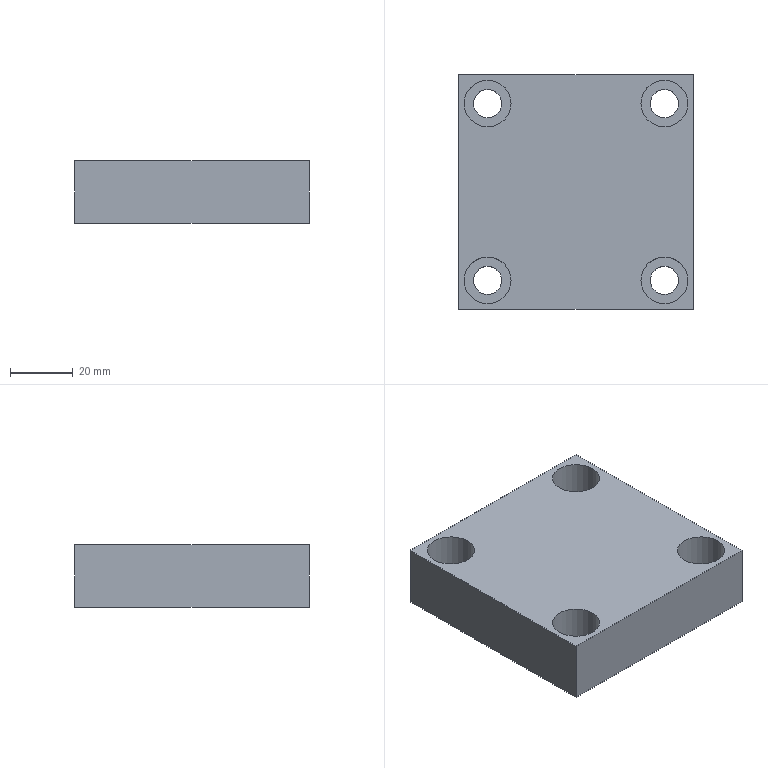Part | NX | features solid 2 | 1 solid | 18 faces | box 75 x 75 x 20 mm | volume 101982 mm3 | plane 10 | cylinder 8 | commonest cylinder face diameters 9 x4 15 x4
STEP:
#1=CARTESIAN_POINT('',(131.25,551.75,290.));
#2=VERTEX_POINT('',#1);
#3=CARTESIAN_POINT('',(126.75,551.75,290.));
#4=DIRECTION('',(0.,0.,1.));
#5=DIRECTION('',(1.,0.,0.));
#6=AXIS2_PLACEMENT_3D('',#3,#4,#5);
#7=CIRCLE('',#6,4.5);
#8=EDGE_CURVE('',#2,#2,#7,.T.);
#9=ORIENTED_EDGE('',*,*,#8,.T.);
#10=EDGE_LOOP('',(#9));
#11=FACE_BOUND('',#10,.T.);
#12=CARTESIAN_POINT('',(187.75,551.75,290.));
#13=VERTEX_POINT('',#12);
#14=CARTESIAN_POINT('',(183.25,551.75,290.));
#15=DIRECTION('',(0.,0.,1.));
#16=DIRECTION('',(1.,0.,0.));
#17=AXIS2_PLACEMENT_3D('',#14,#15,#16);
#18=CIRCLE('',#17,4.5);
#19=EDGE_CURVE('',#13,#13,#18,.T.);
#20=ORIENTED_EDGE('',*,*,#19,.T.);
#21=EDGE_LOOP('',(#20));
#22=FACE_BOUND('',#21,.T.);
#23=CARTESIAN_POINT('',(187.75,608.25,290.));
#24=VERTEX_POINT('',#23);
#25=CARTESIAN_POINT('',(183.25,608.25,290.));
#26=DIRECTION('',(0.,0.,1.));
#27=DIRECTION('',(1.,0.,0.));
#28=AXIS2_PLACEMENT_3D('',#25,#26,#27);
#29=CIRCLE('',#28,4.5);
#30=EDGE_CURVE('',#24,#24,#29,.T.);
#31=ORIENTED_EDGE('',*,*,#30,.T.);
#32=EDGE_LOOP('',(#31));
#33=FACE_BOUND('',#32,.T.);
#34=CARTESIAN_POINT('',(131.25,608.25,290.));
#35=VERTEX_POINT('',#34);
#36=CARTESIAN_POINT('',(126.75,608.25,290.));
#37=DIRECTION('',(0.,0.,1.));
#38=DIRECTION('',(1.,0.,0.));
#39=AXIS2_PLACEMENT_3D('',#36,#37,#38);
#40=CIRCLE('',#39,4.5);
#41=EDGE_CURVE('',#35,#35,#40,.T.);
#42=ORIENTED_EDGE('',*,*,#41,.T.);
#43=EDGE_LOOP('',(#42));
#44=FACE_BOUND('',#43,.T.);
#45=CARTESIAN_POINT('',(192.5,542.5,290.));
#46=VERTEX_POINT('',#45);
#47=CARTESIAN_POINT('',(117.5,542.5,290.));
#48=VERTEX_POINT('',#47);
#49=CARTESIAN_POINT('',(192.5,542.5,290.));
#50=DIRECTION('',(1.,0.,0.));
#51=VECTOR('',#50,1000.);
#52=LINE('',#49,#51);
#53=EDGE_CURVE('',#46,#48,#52,.F.);
#54=ORIENTED_EDGE('',*,*,#53,.T.);
#55=CARTESIAN_POINT('',(117.5,617.5,290.));
#56=VERTEX_POINT('',#55);
#57=CARTESIAN_POINT('',(117.5,630.,290.));
#58=DIRECTION('',(0.,-1.,0.));
#59=VECTOR('',#58,1000.);
#60=LINE('',#57,#59);
#61=EDGE_CURVE('',#56,#48,#60,.T.);
#62=ORIENTED_EDGE('',*,*,#61,.F.);
#63=CARTESIAN_POINT('',(192.5,617.5,290.));
#64=VERTEX_POINT('',#63);
#65=CARTESIAN_POINT('',(192.5,617.5,290.));
#66=DIRECTION('',(-1.,0.,0.));
#67=VECTOR('',#66,1000.);
#68=LINE('',#65,#67);
#69=EDGE_CURVE('',#64,#56,#68,.T.);
#70=ORIENTED_EDGE('',*,*,#69,.F.);
#71=CARTESIAN_POINT('',(192.5,630.,290.));
#72=DIRECTION('',(0.,1.,0.));
#73=VECTOR('',#72,1000.);
#74=LINE('',#71,#73);
#75=EDGE_CURVE('',#64,#46,#74,.F.);
#76=ORIENTED_EDGE('',*,*,#75,.T.);
#77=EDGE_LOOP('',(#54,#62,#70,#76));
#78=FACE_BOUND('',#77,.T.);
#79=CARTESIAN_POINT('',(192.5,630.,290.));
#80=DIRECTION('',(0.,0.,-1.));
#81=DIRECTION('',(1.,0.,0.));
#82=AXIS2_PLACEMENT_3D('',#79,#80,#81);
#83=PLANE('',#82);
#84=ADVANCED_FACE('',(#11,#22,#33,#44,#78),#83,.T.);
#85=CARTESIAN_POINT('',(117.5,617.5,310.));
#86=VERTEX_POINT('',#85);
#87=CARTESIAN_POINT('',(117.5,617.5,290.));
#88=DIRECTION('',(0.,0.,1.));
#89=VECTOR('',#88,1000.);
#90=LINE('',#87,#89);
#91=EDGE_CURVE('',#56,#86,#90,.T.);
#92=ORIENTED_EDGE('',*,*,#91,.T.);
#93=CARTESIAN_POINT('',(192.5,617.5,310.));
#94=VERTEX_POINT('',#93);
#95=CARTESIAN_POINT('',(192.5,617.5,310.));
#96=DIRECTION('',(-1.,0.,0.));
#97=VECTOR('',#96,1000.);
#98=LINE('',#95,#97);
#99=EDGE_CURVE('',#94,#86,#98,.T.);
#100=ORIENTED_EDGE('',*,*,#99,.F.);
#101=CARTESIAN_POINT('',(192.5,617.5,290.));
#102=DIRECTION('',(0.,0.,-1.));
#103=VECTOR('',#102,1000.);
#104=LINE('',#101,#103);
#105=EDGE_CURVE('',#64,#94,#104,.F.);
#106=ORIENTED_EDGE('',*,*,#105,.F.);
#107=ORIENTED_EDGE('',*,*,#69,.T.);
#108=EDGE_LOOP('',(#92,#100,#106,#107));
#109=FACE_BOUND('',#108,.T.);
#110=CARTESIAN_POINT('',(192.5,617.5,290.));
#111=DIRECTION('',(0.,1.,0.));
#112=DIRECTION('',(-1.,0.,0.));
#113=AXIS2_PLACEMENT_3D('',#110,#111,#112);
#114=PLANE('',#113);
#115=ADVANCED_FACE('',(#109),#114,.T.);
#116=ORIENTED_EDGE('',*,*,#105,.T.);
#117=CARTESIAN_POINT('',(192.5,542.5,310.));
#118=VERTEX_POINT('',#117);
#119=CARTESIAN_POINT('',(192.5,630.,310.));
#120=DIRECTION('',(0.,1.,0.));
#121=VECTOR('',#120,1000.);
#122=LINE('',#119,#121);
#123=EDGE_CURVE('',#94,#118,#122,.F.);
#124=ORIENTED_EDGE('',*,*,#123,.T.);
#125=CARTESIAN_POINT('',(192.5,542.5,290.));
#126=DIRECTION('',(0.,0.,1.));
#127=VECTOR('',#126,1000.);
#128=LINE('',#125,#127);
#129=EDGE_CURVE('',#46,#118,#128,.T.);
#130=ORIENTED_EDGE('',*,*,#129,.F.);
#131=ORIENTED_EDGE('',*,*,#75,.F.);
#132=EDGE_LOOP('',(#116,#124,#130,#131));
#133=FACE_BOUND('',#132,.T.);
#134=CARTESIAN_POINT('',(192.5,630.,290.));
#135=DIRECTION('',(-1.,0.,0.));
#136=DIRECTION('',(0.,-1.,0.));
#137=AXIS2_PLACEMENT_3D('',#134,#135,#136);
#138=PLANE('',#137);
#139=ADVANCED_FACE('',(#133),#138,.F.);
#140=ORIENTED_EDGE('',*,*,#129,.T.);
#141=CARTESIAN_POINT('',(117.5,542.5,310.));
#142=VERTEX_POINT('',#141);
#143=CARTESIAN_POINT('',(192.5,542.5,310.));
#144=DIRECTION('',(1.,0.,0.));
#145=VECTOR('',#144,1000.);
#146=LINE('',#143,#145);
#147=EDGE_CURVE('',#118,#142,#146,.F.);
#148=ORIENTED_EDGE('',*,*,#147,.T.);
#149=CARTESIAN_POINT('',(117.5,542.5,290.));
#150=DIRECTION('',(0.,0.,-1.));
#151=VECTOR('',#150,1000.);
#152=LINE('',#149,#151);
#153=EDGE_CURVE('',#48,#142,#152,.F.);
#154=ORIENTED_EDGE('',*,*,#153,.F.);
#155=ORIENTED_EDGE('',*,*,#53,.F.);
#156=EDGE_LOOP('',(#140,#148,#154,#155));
#157=FACE_BOUND('',#156,.T.);
#158=CARTESIAN_POINT('',(192.5,542.5,290.));
#159=DIRECTION('',(0.,1.,0.));
#160=DIRECTION('',(-1.,0.,0.));
#161=AXIS2_PLACEMENT_3D('',#158,#159,#160);
#162=PLANE('',#161);
#163=ADVANCED_FACE('',(#157),#162,.F.);
#164=ORIENTED_EDGE('',*,*,#61,.T.);
#165=ORIENTED_EDGE('',*,*,#153,.T.);
#166=CARTESIAN_POINT('',(117.5,630.,310.));
#167=DIRECTION('',(0.,-1.,0.));
#168=VECTOR('',#167,1000.);
#169=LINE('',#166,#168);
#170=EDGE_CURVE('',#86,#142,#169,.T.);
#171=ORIENTED_EDGE('',*,*,#170,.F.);
#172=ORIENTED_EDGE('',*,*,#91,.F.);
#173=EDGE_LOOP('',(#164,#165,#171,#172));
#174=FACE_BOUND('',#173,.T.);
#175=CARTESIAN_POINT('',(117.5,630.,290.));
#176=DIRECTION('',(-1.,0.,0.));
#177=DIRECTION('',(0.,-1.,0.));
#178=AXIS2_PLACEMENT_3D('',#175,#176,#177);
#179=PLANE('',#178);
#180=ADVANCED_FACE('',(#174),#179,.T.);
#181=CARTESIAN_POINT('',(134.25,551.75,310.));
#182=VERTEX_POINT('',#181);
#183=CARTESIAN_POINT('',(126.75,551.75,310.));
#184=DIRECTION('',(0.,0.,1.));
#185=DIRECTION('',(1.,0.,0.));
#186=AXIS2_PLACEMENT_3D('',#183,#184,#185);
#187=CIRCLE('',#186,7.5);
#188=EDGE_CURVE('',#182,#182,#187,.T.);
#189=ORIENTED_EDGE('',*,*,#188,.F.);
#190=EDGE_LOOP('',(#189));
#191=FACE_BOUND('',#190,.T.);
#192=CARTESIAN_POINT('',(190.75,551.75,310.));
#193=VERTEX_POINT('',#192);
#194=CARTESIAN_POINT('',(183.25,551.75,310.));
#195=DIRECTION('',(0.,0.,1.));
#196=DIRECTION('',(1.,0.,0.));
#197=AXIS2_PLACEMENT_3D('',#194,#195,#196);
#198=CIRCLE('',#197,7.5);
#199=EDGE_CURVE('',#193,#193,#198,.T.);
#200=ORIENTED_EDGE('',*,*,#199,.F.);
#201=EDGE_LOOP('',(#200));
#202=FACE_BOUND('',#201,.T.);
#203=CARTESIAN_POINT('',(190.75,608.25,310.));
#204=VERTEX_POINT('',#203);
#205=CARTESIAN_POINT('',(183.25,608.25,310.));
#206=DIRECTION('',(0.,0.,1.));
#207=DIRECTION('',(1.,0.,0.));
#208=AXIS2_PLACEMENT_3D('',#205,#206,#207);
#209=CIRCLE('',#208,7.5);
#210=EDGE_CURVE('',#204,#204,#209,.T.);
#211=ORIENTED_EDGE('',*,*,#210,.F.);
#212=EDGE_LOOP('',(#211));
#213=FACE_BOUND('',#212,.T.);
#214=CARTESIAN_POINT('',(134.25,608.25,310.));
#215=VERTEX_POINT('',#214);
#216=CARTESIAN_POINT('',(126.75,608.25,310.));
#217=DIRECTION('',(0.,0.,1.));
#218=DIRECTION('',(1.,0.,0.));
#219=AXIS2_PLACEMENT_3D('',#216,#217,#218);
#220=CIRCLE('',#219,7.5);
#221=EDGE_CURVE('',#215,#215,#220,.T.);
#222=ORIENTED_EDGE('',*,*,#221,.F.);
#223=EDGE_LOOP('',(#222));
#224=FACE_BOUND('',#223,.T.);
#225=ORIENTED_EDGE('',*,*,#147,.F.);
#226=ORIENTED_EDGE('',*,*,#123,.F.);
#227=ORIENTED_EDGE('',*,*,#99,.T.);
#228=ORIENTED_EDGE('',*,*,#170,.T.);
#229=EDGE_LOOP('',(#225,#226,#227,#228));
#230=FACE_BOUND('',#229,.T.);
#231=CARTESIAN_POINT('',(192.5,630.,310.));
#232=DIRECTION('',(0.,0.,-1.));
#233=DIRECTION('',(1.,0.,0.));
#234=AXIS2_PLACEMENT_3D('',#231,#232,#233);
#235=PLANE('',#234);
#236=ADVANCED_FACE('',(#191,#202,#213,#224,#230),#235,.F.);
#237=CARTESIAN_POINT('',(134.25,608.25,298.));
#238=VERTEX_POINT('',#237);
#239=CARTESIAN_POINT('',(126.75,608.25,298.));
#240=DIRECTION('',(0.,0.,-1.));
#241=DIRECTION('',(1.,0.,0.));
#242=AXIS2_PLACEMENT_3D('',#239,#240,#241);
#243=CIRCLE('',#242,7.5);
#244=EDGE_CURVE('',#238,#238,#243,.T.);
#245=ORIENTED_EDGE('',*,*,#244,.T.);
#246=EDGE_LOOP('',(#245));
#247=FACE_BOUND('',#246,.T.);
#248=ORIENTED_EDGE('',*,*,#221,.T.);
#249=EDGE_LOOP('',(#248));
#250=FACE_BOUND('',#249,.T.);
#251=CARTESIAN_POINT('',(126.75,608.25,298.));
#252=DIRECTION('',(0.,0.,1.));
#253=DIRECTION('',(-1.,0.,0.));
#254=AXIS2_PLACEMENT_3D('',#251,#252,#253);
#255=CYLINDRICAL_SURFACE('',#254,7.5);
#256=ADVANCED_FACE('',(#247,#250),#255,.F.);
#257=CARTESIAN_POINT('',(122.25,608.25,298.));
#258=VERTEX_POINT('',#257);
#259=CARTESIAN_POINT('',(126.75,608.25,298.));
#260=DIRECTION('',(0.,0.,-1.));
#261=DIRECTION('',(-1.,0.,0.));
#262=AXIS2_PLACEMENT_3D('',#259,#260,#261);
#263=CIRCLE('',#262,4.5);
#264=EDGE_CURVE('',#258,#258,#263,.T.);
#265=ORIENTED_EDGE('',*,*,#264,.T.);
#266=EDGE_LOOP('',(#265));
#267=FACE_BOUND('',#266,.T.);
#268=ORIENTED_EDGE('',*,*,#244,.F.);
#269=EDGE_LOOP('',(#268));
#270=FACE_BOUND('',#269,.T.);
#271=CARTESIAN_POINT('',(126.75,608.25,298.));
#272=DIRECTION('',(0.,0.,1.));
#273=DIRECTION('',(-1.,0.,0.));
#274=AXIS2_PLACEMENT_3D('',#271,#272,#273);
#275=PLANE('',#274);
#276=ADVANCED_FACE('',(#267,#270),#275,.T.);
#277=ORIENTED_EDGE('',*,*,#41,.F.);
#278=EDGE_LOOP('',(#277));
#279=FACE_BOUND('',#278,.T.);
#280=ORIENTED_EDGE('',*,*,#264,.F.);
#281=EDGE_LOOP('',(#280));
#282=FACE_BOUND('',#281,.T.);
#283=CARTESIAN_POINT('',(126.75,608.25,278.));
#284=DIRECTION('',(0.,0.,1.));
#285=DIRECTION('',(-1.,0.,0.));
#286=AXIS2_PLACEMENT_3D('',#283,#284,#285);
#287=CYLINDRICAL_SURFACE('',#286,4.5);
#288=ADVANCED_FACE('',(#279,#282),#287,.F.);
#289=CARTESIAN_POINT('',(190.75,608.25,298.));
#290=VERTEX_POINT('',#289);
#291=CARTESIAN_POINT('',(183.25,608.25,298.));
#292=DIRECTION('',(0.,0.,-1.));
#293=DIRECTION('',(1.,0.,0.));
#294=AXIS2_PLACEMENT_3D('',#291,#292,#293);
#295=CIRCLE('',#294,7.5);
#296=EDGE_CURVE('',#290,#290,#295,.T.);
#297=ORIENTED_EDGE('',*,*,#296,.T.);
#298=EDGE_LOOP('',(#297));
#299=FACE_BOUND('',#298,.T.);
#300=ORIENTED_EDGE('',*,*,#210,.T.);
#301=EDGE_LOOP('',(#300));
#302=FACE_BOUND('',#301,.T.);
#303=CARTESIAN_POINT('',(183.25,608.25,298.));
#304=DIRECTION('',(0.,0.,1.));
#305=DIRECTION('',(-1.,0.,0.));
#306=AXIS2_PLACEMENT_3D('',#303,#304,#305);
#307=CYLINDRICAL_SURFACE('',#306,7.5);
#308=ADVANCED_FACE('',(#299,#302),#307,.F.);
#309=CARTESIAN_POINT('',(178.75,608.25,298.));
#310=VERTEX_POINT('',#309);
#311=CARTESIAN_POINT('',(183.25,608.25,298.));
#312=DIRECTION('',(0.,0.,-1.));
#313=DIRECTION('',(-1.,0.,0.));
#314=AXIS2_PLACEMENT_3D('',#311,#312,#313);
#315=CIRCLE('',#314,4.5);
#316=EDGE_CURVE('',#310,#310,#315,.T.);
#317=ORIENTED_EDGE('',*,*,#316,.T.);
#318=EDGE_LOOP('',(#317));
#319=FACE_BOUND('',#318,.T.);
#320=ORIENTED_EDGE('',*,*,#296,.F.);
#321=EDGE_LOOP('',(#320));
#322=FACE_BOUND('',#321,.T.);
#323=CARTESIAN_POINT('',(183.25,608.25,298.));
#324=DIRECTION('',(0.,0.,1.));
#325=DIRECTION('',(-1.,0.,0.));
#326=AXIS2_PLACEMENT_3D('',#323,#324,#325);
#327=PLANE('',#326);
#328=ADVANCED_FACE('',(#319,#322),#327,.T.);
#329=ORIENTED_EDGE('',*,*,#30,.F.);
#330=EDGE_LOOP('',(#329));
#331=FACE_BOUND('',#330,.T.);
#332=ORIENTED_EDGE('',*,*,#316,.F.);
#333=EDGE_LOOP('',(#332));
#334=FACE_BOUND('',#333,.T.);
#335=CARTESIAN_POINT('',(183.25,608.25,278.));
#336=DIRECTION('',(0.,0.,1.));
#337=DIRECTION('',(-1.,0.,0.));
#338=AXIS2_PLACEMENT_3D('',#335,#336,#337);
#339=CYLINDRICAL_SURFACE('',#338,4.5);
#340=ADVANCED_FACE('',(#331,#334),#339,.F.);
#341=CARTESIAN_POINT('',(190.75,551.75,298.));
#342=VERTEX_POINT('',#341);
#343=CARTESIAN_POINT('',(183.25,551.75,298.));
#344=DIRECTION('',(0.,0.,-1.));
#345=DIRECTION('',(1.,0.,0.));
#346=AXIS2_PLACEMENT_3D('',#343,#344,#345);
#347=CIRCLE('',#346,7.5);
#348=EDGE_CURVE('',#342,#342,#347,.T.);
#349=ORIENTED_EDGE('',*,*,#348,.T.);
#350=EDGE_LOOP('',(#349));
#351=FACE_BOUND('',#350,.T.);
#352=ORIENTED_EDGE('',*,*,#199,.T.);
#353=EDGE_LOOP('',(#352));
#354=FACE_BOUND('',#353,.T.);
#355=CARTESIAN_POINT('',(183.25,551.75,298.));
#356=DIRECTION('',(0.,0.,1.));
#357=DIRECTION('',(-1.,0.,0.));
#358=AXIS2_PLACEMENT_3D('',#355,#356,#357);
#359=CYLINDRICAL_SURFACE('',#358,7.5);
#360=ADVANCED_FACE('',(#351,#354),#359,.F.);
#361=CARTESIAN_POINT('',(178.75,551.75,298.));
#362=VERTEX_POINT('',#361);
#363=CARTESIAN_POINT('',(183.25,551.75,298.));
#364=DIRECTION('',(0.,0.,-1.));
#365=DIRECTION('',(-1.,0.,0.));
#366=AXIS2_PLACEMENT_3D('',#363,#364,#365);
#367=CIRCLE('',#366,4.5);
#368=EDGE_CURVE('',#362,#362,#367,.T.);
#369=ORIENTED_EDGE('',*,*,#368,.T.);
#370=EDGE_LOOP('',(#369));
#371=FACE_BOUND('',#370,.T.);
#372=ORIENTED_EDGE('',*,*,#348,.F.);
#373=EDGE_LOOP('',(#372));
#374=FACE_BOUND('',#373,.T.);
#375=CARTESIAN_POINT('',(183.25,551.75,298.));
#376=DIRECTION('',(0.,0.,1.));
#377=DIRECTION('',(-1.,0.,0.));
#378=AXIS2_PLACEMENT_3D('',#375,#376,#377);
#379=PLANE('',#378);
#380=ADVANCED_FACE('',(#371,#374),#379,.T.);
#381=ORIENTED_EDGE('',*,*,#19,.F.);
#382=EDGE_LOOP('',(#381));
#383=FACE_BOUND('',#382,.T.);
#384=ORIENTED_EDGE('',*,*,#368,.F.);
#385=EDGE_LOOP('',(#384));
#386=FACE_BOUND('',#385,.T.);
#387=CARTESIAN_POINT('',(183.25,551.75,278.));
#388=DIRECTION('',(0.,0.,1.));
#389=DIRECTION('',(-1.,0.,0.));
#390=AXIS2_PLACEMENT_3D('',#387,#388,#389);
#391=CYLINDRICAL_SURFACE('',#390,4.5);
#392=ADVANCED_FACE('',(#383,#386),#391,.F.);
#393=CARTESIAN_POINT('',(134.25,551.75,298.));
#394=VERTEX_POINT('',#393);
#395=CARTESIAN_POINT('',(126.75,551.75,298.));
#396=DIRECTION('',(0.,0.,-1.));
#397=DIRECTION('',(1.,0.,0.));
#398=AXIS2_PLACEMENT_3D('',#395,#396,#397);
#399=CIRCLE('',#398,7.5);
#400=EDGE_CURVE('',#394,#394,#399,.T.);
#401=ORIENTED_EDGE('',*,*,#400,.T.);
#402=EDGE_LOOP('',(#401));
#403=FACE_BOUND('',#402,.T.);
#404=ORIENTED_EDGE('',*,*,#188,.T.);
#405=EDGE_LOOP('',(#404));
#406=FACE_BOUND('',#405,.T.);
#407=CARTESIAN_POINT('',(126.75,551.75,298.));
#408=DIRECTION('',(0.,0.,1.));
#409=DIRECTION('',(-1.,0.,0.));
#410=AXIS2_PLACEMENT_3D('',#407,#408,#409);
#411=CYLINDRICAL_SURFACE('',#410,7.5);
#412=ADVANCED_FACE('',(#403,#406),#411,.F.);
#413=CARTESIAN_POINT('',(122.25,551.75,298.));
#414=VERTEX_POINT('',#413);
#415=CARTESIAN_POINT('',(126.75,551.75,298.));
#416=DIRECTION('',(0.,0.,-1.));
#417=DIRECTION('',(-1.,0.,0.));
#418=AXIS2_PLACEMENT_3D('',#415,#416,#417);
#419=CIRCLE('',#418,4.5);
#420=EDGE_CURVE('',#414,#414,#419,.T.);
#421=ORIENTED_EDGE('',*,*,#420,.T.);
#422=EDGE_LOOP('',(#421));
#423=FACE_BOUND('',#422,.T.);
#424=ORIENTED_EDGE('',*,*,#400,.F.);
#425=EDGE_LOOP('',(#424));
#426=FACE_BOUND('',#425,.T.);
#427=CARTESIAN_POINT('',(126.75,551.75,298.));
#428=DIRECTION('',(0.,0.,1.));
#429=DIRECTION('',(-1.,0.,0.));
#430=AXIS2_PLACEMENT_3D('',#427,#428,#429);
#431=PLANE('',#430);
#432=ADVANCED_FACE('',(#423,#426),#431,.T.);
#433=ORIENTED_EDGE('',*,*,#8,.F.);
#434=EDGE_LOOP('',(#433));
#435=FACE_BOUND('',#434,.T.);
#436=ORIENTED_EDGE('',*,*,#420,.F.);
#437=EDGE_LOOP('',(#436));
#438=FACE_BOUND('',#437,.T.);
#439=CARTESIAN_POINT('',(126.75,551.75,278.));
#440=DIRECTION('',(0.,0.,1.));
#441=DIRECTION('',(-1.,0.,0.));
#442=AXIS2_PLACEMENT_3D('',#439,#440,#441);
#443=CYLINDRICAL_SURFACE('',#442,4.5);
#444=ADVANCED_FACE('',(#435,#438),#443,.F.);
#445=CLOSED_SHELL('',(#84,#115,#139,#163,#180,#236,#256,#276,#288,#308,#328,#340,#360,#380,#392,#412,#432,#444));
#446=MANIFOLD_SOLID_BREP('',#445);
#447=(LENGTH_UNIT()NAMED_UNIT(*)SI_UNIT(.MILLI.,.METRE.));
#448=UNCERTAINTY_MEASURE_WITH_UNIT(LENGTH_MEASURE(0.00001),#447,'','');
#449=(NAMED_UNIT(*)PLANE_ANGLE_UNIT()SI_UNIT($,.RADIAN.));
#450=(NAMED_UNIT(*)SI_UNIT($,.STERADIAN.)SOLID_ANGLE_UNIT());
#451=(GEOMETRIC_REPRESENTATION_CONTEXT(3)GLOBAL_UNCERTAINTY_ASSIGNED_CONTEXT((#448))GLOBAL_UNIT_ASSIGNED_CONTEXT((#447,#449,#450))REPRESENTATION_CONTEXT('',''));
#452=ADVANCED_BREP_SHAPE_REPRESENTATION('',(#446),#451);